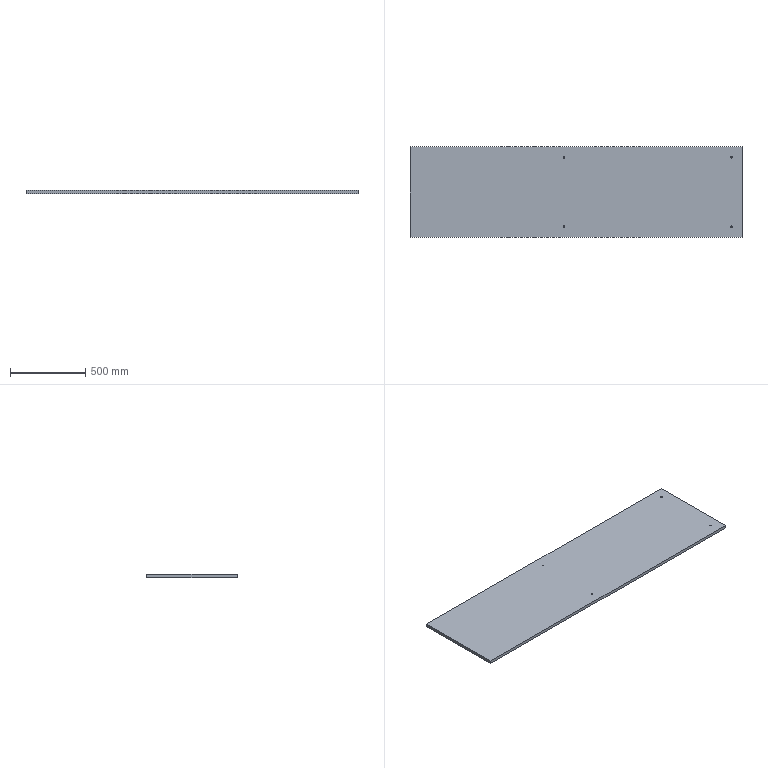Part | STEP file | B1-003 | 1 solid | 14 faces | box 2200 x 600 x 20 mm | volume 26393073 mm3 | cylinder 8 | plane 6 | commonest cylinder face diameters 10.5 x8
STEP:
#1=CARTESIAN_POINT('',(0.,0.,0.));
#2=DIRECTION('',(0.,0.,1.));
#3=DIRECTION('',(1.,0.,0.));
#4=AXIS2_PLACEMENT_3D('',#1,#2,#3);
#5=CARTESIAN_POINT('',(-85.25,230.,10.));
#6=VERTEX_POINT('',#5);
#7=CARTESIAN_POINT('',(-85.25,230.,-10.));
#8=VERTEX_POINT('',#7);
#9=CARTESIAN_POINT('',(-85.25,230.,24.849));
#10=DIRECTION('',(0.,0.,-1.));
#11=VECTOR('',#10,1.);
#12=LINE('',#9,#11);
#13=CARTESIAN_POINT('',(-80.,230.,24.849));
#14=DIRECTION('',(0.,0.,-1.));
#15=DIRECTION('',(-1.,0.,0.));
#16=AXIS2_PLACEMENT_3D('',#13,#14,#15);
#17=CYLINDRICAL_SURFACE('',#16,5.25);
#18=CARTESIAN_POINT('',(6.283,0.));
#19=DIRECTION('',(0.,1.));
#20=VECTOR('',#19,1.);
#21=LINE('',#18,#20);
#22=(GEOMETRIC_REPRESENTATION_CONTEXT(2)PARAMETRIC_REPRESENTATION_CONTEXT()REPRESENTATION_CONTEXT('',''));
#23=DEFINITIONAL_REPRESENTATION('',(#21),#22);
#24=PCURVE('',#17,#23);
#25=CARTESIAN_POINT('',(-80.,230.,24.849));
#26=DIRECTION('',(0.,0.,-1.));
#27=DIRECTION('',(-1.,0.,0.));
#28=AXIS2_PLACEMENT_3D('',#25,#26,#27);
#29=CYLINDRICAL_SURFACE('',#28,5.25);
#30=CARTESIAN_POINT('',(0.,0.));
#31=DIRECTION('',(0.,1.));
#32=VECTOR('',#31,1.);
#33=LINE('',#30,#32);
#34=(GEOMETRIC_REPRESENTATION_CONTEXT(2)PARAMETRIC_REPRESENTATION_CONTEXT()REPRESENTATION_CONTEXT('',''));
#35=DEFINITIONAL_REPRESENTATION('',(#33),#34);
#36=PCURVE('',#29,#35);
#37=SURFACE_CURVE('',#12,(#24,#36),.PCURVE_S1.);
#38=EDGE_CURVE('',#6,#8,#37,.T.);
#39=ORIENTED_EDGE('',*,*,#38,.T.);
#40=CARTESIAN_POINT('',(-74.75,230.,-10.));
#41=VERTEX_POINT('',#40);
#42=CARTESIAN_POINT('',(-80.,230.,-10.));
#43=DIRECTION('',(0.,0.,-1.));
#44=DIRECTION('',(-1.,0.,0.));
#45=AXIS2_PLACEMENT_3D('',#42,#43,#44);
#46=CIRCLE('',#45,5.25);
#47=CARTESIAN_POINT('',(0.,34.849));
#48=DIRECTION('',(1.,0.));
#49=VECTOR('',#48,1.);
#50=LINE('',#47,#49);
#51=(GEOMETRIC_REPRESENTATION_CONTEXT(2)PARAMETRIC_REPRESENTATION_CONTEXT()REPRESENTATION_CONTEXT('',''));
#52=DEFINITIONAL_REPRESENTATION('',(#50),#51);
#53=PCURVE('',#17,#52);
#54=CARTESIAN_POINT('',(0.,0.,-10.));
#55=DIRECTION('',(0.,0.,1.));
#56=DIRECTION('',(1.,0.,0.));
#57=AXIS2_PLACEMENT_3D('',#54,#55,#56);
#58=PLANE('',#57);
#59=CARTESIAN_POINT('',(-85.25,230.));
#60=CARTESIAN_POINT('',(-85.25,239.093));
#61=CARTESIAN_POINT('',(-77.375,234.547));
#62=CARTESIAN_POINT('',(-69.5,230.));
#63=CARTESIAN_POINT('',(-77.375,225.453));
#64=CARTESIAN_POINT('',(-85.25,220.907));
#65=CARTESIAN_POINT('',(-85.25,230.));
#66=(BOUNDED_CURVE()B_SPLINE_CURVE(2,(#59,#60,#61,#62,#63,#64,#65),.UNSPECIFIED.,.T.,.F.)B_SPLINE_CURVE_WITH_KNOTS((1,2,2,2,2,1),(-2.094,0.,2.094,4.189,6.283,8.378),.UNSPECIFIED.)CURVE()GEOMETRIC_REPRESENTATION_ITEM()RATIONAL_B_SPLINE_CURVE((1.,0.5,1.,0.5,1.,0.5,1.))REPRESENTATION_ITEM(''));
#67=(GEOMETRIC_REPRESENTATION_CONTEXT(2)PARAMETRIC_REPRESENTATION_CONTEXT()REPRESENTATION_CONTEXT('',''));
#68=DEFINITIONAL_REPRESENTATION('',(#66),#67);
#69=PCURVE('',#58,#68);
#70=SURFACE_CURVE('',#46,(#53,#69),.PCURVE_S1.);
#71=EDGE_CURVE('',#41,#8,#70,.T.);
#72=ORIENTED_EDGE('',*,*,#71,.F.);
#73=CARTESIAN_POINT('',(-74.75,230.,10.));
#74=VERTEX_POINT('',#73);
#75=CARTESIAN_POINT('',(-74.75,230.,24.849));
#76=DIRECTION('',(0.,0.,-1.));
#77=VECTOR('',#76,1.);
#78=LINE('',#75,#77);
#79=CARTESIAN_POINT('',(3.142,0.));
#80=DIRECTION('',(0.,1.));
#81=VECTOR('',#80,1.);
#82=LINE('',#79,#81);
#83=(GEOMETRIC_REPRESENTATION_CONTEXT(2)PARAMETRIC_REPRESENTATION_CONTEXT()REPRESENTATION_CONTEXT('',''));
#84=DEFINITIONAL_REPRESENTATION('',(#82),#83);
#85=PCURVE('',#17,#84);
#86=CARTESIAN_POINT('',(3.142,0.));
#87=DIRECTION('',(0.,1.));
#88=VECTOR('',#87,1.);
#89=LINE('',#86,#88);
#90=(GEOMETRIC_REPRESENTATION_CONTEXT(2)PARAMETRIC_REPRESENTATION_CONTEXT()REPRESENTATION_CONTEXT('',''));
#91=DEFINITIONAL_REPRESENTATION('',(#89),#90);
#92=PCURVE('',#29,#91);
#93=SURFACE_CURVE('',#78,(#85,#92),.PCURVE_S1.);
#94=EDGE_CURVE('',#74,#41,#93,.T.);
#95=ORIENTED_EDGE('',*,*,#94,.F.);
#96=CARTESIAN_POINT('',(-80.,230.,10.));
#97=DIRECTION('',(0.,0.,-1.));
#98=DIRECTION('',(1.,0.,0.));
#99=AXIS2_PLACEMENT_3D('',#96,#97,#98);
#100=CIRCLE('',#99,5.25);
#101=CARTESIAN_POINT('',(3.142,14.849));
#102=DIRECTION('',(1.,0.));
#103=VECTOR('',#102,1.);
#104=LINE('',#101,#103);
#105=(GEOMETRIC_REPRESENTATION_CONTEXT(2)PARAMETRIC_REPRESENTATION_CONTEXT()REPRESENTATION_CONTEXT('',''));
#106=DEFINITIONAL_REPRESENTATION('',(#104),#105);
#107=PCURVE('',#17,#106);
#108=CARTESIAN_POINT('',(0.,0.,10.));
#109=DIRECTION('',(0.,0.,1.));
#110=DIRECTION('',(1.,0.,0.));
#111=AXIS2_PLACEMENT_3D('',#108,#109,#110);
#112=PLANE('',#111);
#113=CARTESIAN_POINT('',(-74.75,230.));
#114=CARTESIAN_POINT('',(-74.75,220.907));
#115=CARTESIAN_POINT('',(-82.625,225.453));
#116=CARTESIAN_POINT('',(-90.5,230.));
#117=CARTESIAN_POINT('',(-82.625,234.547));
#118=CARTESIAN_POINT('',(-74.75,239.093));
#119=CARTESIAN_POINT('',(-74.75,230.));
#120=(BOUNDED_CURVE()B_SPLINE_CURVE(2,(#113,#114,#115,#116,#117,#118,#119),.UNSPECIFIED.,.T.,.F.)B_SPLINE_CURVE_WITH_KNOTS((1,2,2,2,2,1),(-2.094,0.,2.094,4.189,6.283,8.378),.UNSPECIFIED.)CURVE()GEOMETRIC_REPRESENTATION_ITEM()RATIONAL_B_SPLINE_CURVE((1.,0.5,1.,0.5,1.,0.5,1.))REPRESENTATION_ITEM(''));
#121=(GEOMETRIC_REPRESENTATION_CONTEXT(2)PARAMETRIC_REPRESENTATION_CONTEXT()REPRESENTATION_CONTEXT('',''));
#122=DEFINITIONAL_REPRESENTATION('',(#120),#121);
#123=PCURVE('',#112,#122);
#124=SURFACE_CURVE('',#100,(#107,#123),.PCURVE_S1.);
#125=EDGE_CURVE('',#74,#6,#124,.T.);
#126=ORIENTED_EDGE('',*,*,#125,.T.);
#127=EDGE_LOOP('',(#39,#72,#95,#126));
#128=FACE_BOUND('',#127,.F.);
#129=ADVANCED_FACE('',(#128),#17,.F.);
#130=CARTESIAN_POINT('',(1024.75,-230.,10.));
#131=VERTEX_POINT('',#130);
#132=CARTESIAN_POINT('',(1024.75,-230.,-10.));
#133=VERTEX_POINT('',#132);
#134=CARTESIAN_POINT('',(1024.75,-230.,24.849));
#135=DIRECTION('',(0.,0.,-1.));
#136=VECTOR('',#135,1.);
#137=LINE('',#134,#136);
#138=CARTESIAN_POINT('',(1030.,-230.,24.849));
#139=DIRECTION('',(0.,0.,-1.));
#140=DIRECTION('',(-1.,0.,0.));
#141=AXIS2_PLACEMENT_3D('',#138,#139,#140);
#142=CYLINDRICAL_SURFACE('',#141,5.25);
#143=CARTESIAN_POINT('',(6.283,0.));
#144=DIRECTION('',(0.,1.));
#145=VECTOR('',#144,1.);
#146=LINE('',#143,#145);
#147=(GEOMETRIC_REPRESENTATION_CONTEXT(2)PARAMETRIC_REPRESENTATION_CONTEXT()REPRESENTATION_CONTEXT('',''));
#148=DEFINITIONAL_REPRESENTATION('',(#146),#147);
#149=PCURVE('',#142,#148);
#150=CARTESIAN_POINT('',(1030.,-230.,24.849));
#151=DIRECTION('',(0.,0.,-1.));
#152=DIRECTION('',(-1.,0.,0.));
#153=AXIS2_PLACEMENT_3D('',#150,#151,#152);
#154=CYLINDRICAL_SURFACE('',#153,5.25);
#155=CARTESIAN_POINT('',(0.,0.));
#156=DIRECTION('',(0.,1.));
#157=VECTOR('',#156,1.);
#158=LINE('',#155,#157);
#159=(GEOMETRIC_REPRESENTATION_CONTEXT(2)PARAMETRIC_REPRESENTATION_CONTEXT()REPRESENTATION_CONTEXT('',''));
#160=DEFINITIONAL_REPRESENTATION('',(#158),#159);
#161=PCURVE('',#154,#160);
#162=SURFACE_CURVE('',#137,(#149,#161),.PCURVE_S1.);
#163=EDGE_CURVE('',#131,#133,#162,.T.);
#164=ORIENTED_EDGE('',*,*,#163,.T.);
#165=CARTESIAN_POINT('',(1035.25,-230.,-10.));
#166=VERTEX_POINT('',#165);
#167=CARTESIAN_POINT('',(1030.,-230.,-10.));
#168=DIRECTION('',(0.,0.,-1.));
#169=DIRECTION('',(-1.,0.,0.));
#170=AXIS2_PLACEMENT_3D('',#167,#168,#169);
#171=CIRCLE('',#170,5.25);
#172=CARTESIAN_POINT('',(0.,34.849));
#173=DIRECTION('',(1.,0.));
#174=VECTOR('',#173,1.);
#175=LINE('',#172,#174);
#176=(GEOMETRIC_REPRESENTATION_CONTEXT(2)PARAMETRIC_REPRESENTATION_CONTEXT()REPRESENTATION_CONTEXT('',''));
#177=DEFINITIONAL_REPRESENTATION('',(#175),#176);
#178=PCURVE('',#142,#177);
#179=CARTESIAN_POINT('',(1024.75,-230.));
#180=CARTESIAN_POINT('',(1024.75,-220.907));
#181=CARTESIAN_POINT('',(1032.625,-225.453));
#182=CARTESIAN_POINT('',(1040.5,-230.));
#183=CARTESIAN_POINT('',(1032.625,-234.547));
#184=CARTESIAN_POINT('',(1024.75,-239.093));
#185=CARTESIAN_POINT('',(1024.75,-230.));
#186=(BOUNDED_CURVE()B_SPLINE_CURVE(2,(#179,#180,#181,#182,#183,#184,#185),.UNSPECIFIED.,.T.,.F.)B_SPLINE_CURVE_WITH_KNOTS((1,2,2,2,2,1),(-2.094,0.,2.094,4.189,6.283,8.378),.UNSPECIFIED.)CURVE()GEOMETRIC_REPRESENTATION_ITEM()RATIONAL_B_SPLINE_CURVE((1.,0.5,1.,0.5,1.,0.5,1.))REPRESENTATION_ITEM(''));
#187=(GEOMETRIC_REPRESENTATION_CONTEXT(2)PARAMETRIC_REPRESENTATION_CONTEXT()REPRESENTATION_CONTEXT('',''));
#188=DEFINITIONAL_REPRESENTATION('',(#186),#187);
#189=PCURVE('',#58,#188);
#190=SURFACE_CURVE('',#171,(#178,#189),.PCURVE_S1.);
#191=EDGE_CURVE('',#166,#133,#190,.T.);
#192=ORIENTED_EDGE('',*,*,#191,.F.);
#193=CARTESIAN_POINT('',(1035.25,-230.,10.));
#194=VERTEX_POINT('',#193);
#195=CARTESIAN_POINT('',(1035.25,-230.,24.849));
#196=DIRECTION('',(0.,0.,-1.));
#197=VECTOR('',#196,1.);
#198=LINE('',#195,#197);
#199=CARTESIAN_POINT('',(3.142,0.));
#200=DIRECTION('',(0.,1.));
#201=VECTOR('',#200,1.);
#202=LINE('',#199,#201);
#203=(GEOMETRIC_REPRESENTATION_CONTEXT(2)PARAMETRIC_REPRESENTATION_CONTEXT()REPRESENTATION_CONTEXT('',''));
#204=DEFINITIONAL_REPRESENTATION('',(#202),#203);
#205=PCURVE('',#142,#204);
#206=CARTESIAN_POINT('',(3.142,0.));
#207=DIRECTION('',(0.,1.));
#208=VECTOR('',#207,1.);
#209=LINE('',#206,#208);
#210=(GEOMETRIC_REPRESENTATION_CONTEXT(2)PARAMETRIC_REPRESENTATION_CONTEXT()REPRESENTATION_CONTEXT('',''));
#211=DEFINITIONAL_REPRESENTATION('',(#209),#210);
#212=PCURVE('',#154,#211);
#213=SURFACE_CURVE('',#198,(#205,#212),.PCURVE_S1.);
#214=EDGE_CURVE('',#194,#166,#213,.T.);
#215=ORIENTED_EDGE('',*,*,#214,.F.);
#216=CARTESIAN_POINT('',(1030.,-230.,10.));
#217=DIRECTION('',(0.,0.,-1.));
#218=DIRECTION('',(1.,0.,0.));
#219=AXIS2_PLACEMENT_3D('',#216,#217,#218);
#220=CIRCLE('',#219,5.25);
#221=CARTESIAN_POINT('',(3.142,14.849));
#222=DIRECTION('',(1.,0.));
#223=VECTOR('',#222,1.);
#224=LINE('',#221,#223);
#225=(GEOMETRIC_REPRESENTATION_CONTEXT(2)PARAMETRIC_REPRESENTATION_CONTEXT()REPRESENTATION_CONTEXT('',''));
#226=DEFINITIONAL_REPRESENTATION('',(#224),#225);
#227=PCURVE('',#142,#226);
#228=CARTESIAN_POINT('',(1035.25,-230.));
#229=CARTESIAN_POINT('',(1035.25,-239.093));
#230=CARTESIAN_POINT('',(1027.375,-234.547));
#231=CARTESIAN_POINT('',(1019.5,-230.));
#232=CARTESIAN_POINT('',(1027.375,-225.453));
#233=CARTESIAN_POINT('',(1035.25,-220.907));
#234=CARTESIAN_POINT('',(1035.25,-230.));
#235=(BOUNDED_CURVE()B_SPLINE_CURVE(2,(#228,#229,#230,#231,#232,#233,#234),.UNSPECIFIED.,.T.,.F.)B_SPLINE_CURVE_WITH_KNOTS((1,2,2,2,2,1),(-2.094,0.,2.094,4.189,6.283,8.378),.UNSPECIFIED.)CURVE()GEOMETRIC_REPRESENTATION_ITEM()RATIONAL_B_SPLINE_CURVE((1.,0.5,1.,0.5,1.,0.5,1.))REPRESENTATION_ITEM(''));
#236=(GEOMETRIC_REPRESENTATION_CONTEXT(2)PARAMETRIC_REPRESENTATION_CONTEXT()REPRESENTATION_CONTEXT('',''));
#237=DEFINITIONAL_REPRESENTATION('',(#235),#236);
#238=PCURVE('',#112,#237);
#239=SURFACE_CURVE('',#220,(#227,#238),.PCURVE_S1.);
#240=EDGE_CURVE('',#194,#131,#239,.T.);
#241=ORIENTED_EDGE('',*,*,#240,.T.);
#242=EDGE_LOOP('',(#164,#192,#215,#241));
#243=FACE_BOUND('',#242,.F.);
#244=ADVANCED_FACE('',(#243),#142,.F.);
#245=CARTESIAN_POINT('',(1024.75,230.,10.));
#246=VERTEX_POINT('',#245);
#247=CARTESIAN_POINT('',(1024.75,230.,-10.));
#248=VERTEX_POINT('',#247);
#249=CARTESIAN_POINT('',(1024.75,230.,24.849));
#250=DIRECTION('',(0.,0.,-1.));
#251=VECTOR('',#250,1.);
#252=LINE('',#249,#251);
#253=CARTESIAN_POINT('',(1030.,230.,24.849));
#254=DIRECTION('',(0.,0.,-1.));
#255=DIRECTION('',(-1.,0.,0.));
#256=AXIS2_PLACEMENT_3D('',#253,#254,#255);
#257=CYLINDRICAL_SURFACE('',#256,5.25);
#258=CARTESIAN_POINT('',(6.283,0.));
#259=DIRECTION('',(0.,1.));
#260=VECTOR('',#259,1.);
#261=LINE('',#258,#260);
#262=(GEOMETRIC_REPRESENTATION_CONTEXT(2)PARAMETRIC_REPRESENTATION_CONTEXT()REPRESENTATION_CONTEXT('',''));
#263=DEFINITIONAL_REPRESENTATION('',(#261),#262);
#264=PCURVE('',#257,#263);
#265=CARTESIAN_POINT('',(1030.,230.,24.849));
#266=DIRECTION('',(0.,0.,-1.));
#267=DIRECTION('',(-1.,0.,0.));
#268=AXIS2_PLACEMENT_3D('',#265,#266,#267);
#269=CYLINDRICAL_SURFACE('',#268,5.25);
#270=CARTESIAN_POINT('',(0.,0.));
#271=DIRECTION('',(0.,1.));
#272=VECTOR('',#271,1.);
#273=LINE('',#270,#272);
#274=(GEOMETRIC_REPRESENTATION_CONTEXT(2)PARAMETRIC_REPRESENTATION_CONTEXT()REPRESENTATION_CONTEXT('',''));
#275=DEFINITIONAL_REPRESENTATION('',(#273),#274);
#276=PCURVE('',#269,#275);
#277=SURFACE_CURVE('',#252,(#264,#276),.PCURVE_S1.);
#278=EDGE_CURVE('',#246,#248,#277,.T.);
#279=ORIENTED_EDGE('',*,*,#278,.T.);
#280=CARTESIAN_POINT('',(1035.25,230.,-10.));
#281=VERTEX_POINT('',#280);
#282=CARTESIAN_POINT('',(1030.,230.,-10.));
#283=DIRECTION('',(0.,0.,-1.));
#284=DIRECTION('',(-1.,0.,0.));
#285=AXIS2_PLACEMENT_3D('',#282,#283,#284);
#286=CIRCLE('',#285,5.25);
#287=CARTESIAN_POINT('',(0.,34.849));
#288=DIRECTION('',(1.,0.));
#289=VECTOR('',#288,1.);
#290=LINE('',#287,#289);
#291=(GEOMETRIC_REPRESENTATION_CONTEXT(2)PARAMETRIC_REPRESENTATION_CONTEXT()REPRESENTATION_CONTEXT('',''));
#292=DEFINITIONAL_REPRESENTATION('',(#290),#291);
#293=PCURVE('',#257,#292);
#294=CARTESIAN_POINT('',(1024.75,230.));
#295=CARTESIAN_POINT('',(1024.75,239.093));
#296=CARTESIAN_POINT('',(1032.625,234.547));
#297=CARTESIAN_POINT('',(1040.5,230.));
#298=CARTESIAN_POINT('',(1032.625,225.453));
#299=CARTESIAN_POINT('',(1024.75,220.907));
#300=CARTESIAN_POINT('',(1024.75,230.));
#301=(BOUNDED_CURVE()B_SPLINE_CURVE(2,(#294,#295,#296,#297,#298,#299,#300),.UNSPECIFIED.,.T.,.F.)B_SPLINE_CURVE_WITH_KNOTS((1,2,2,2,2,1),(-2.094,0.,2.094,4.189,6.283,8.378),.UNSPECIFIED.)CURVE()GEOMETRIC_REPRESENTATION_ITEM()RATIONAL_B_SPLINE_CURVE((1.,0.5,1.,0.5,1.,0.5,1.))REPRESENTATION_ITEM(''));
#302=(GEOMETRIC_REPRESENTATION_CONTEXT(2)PARAMETRIC_REPRESENTATION_CONTEXT()REPRESENTATION_CONTEXT('',''));
#303=DEFINITIONAL_REPRESENTATION('',(#301),#302);
#304=PCURVE('',#58,#303);
#305=SURFACE_CURVE('',#286,(#293,#304),.PCURVE_S1.);
#306=EDGE_CURVE('',#281,#248,#305,.T.);
#307=ORIENTED_EDGE('',*,*,#306,.F.);
#308=CARTESIAN_POINT('',(1035.25,230.,10.));
#309=VERTEX_POINT('',#308);
#310=CARTESIAN_POINT('',(1035.25,230.,24.849));
#311=DIRECTION('',(0.,0.,-1.));
#312=VECTOR('',#311,1.);
#313=LINE('',#310,#312);
#314=CARTESIAN_POINT('',(3.142,0.));
#315=DIRECTION('',(0.,1.));
#316=VECTOR('',#315,1.);
#317=LINE('',#314,#316);
#318=(GEOMETRIC_REPRESENTATION_CONTEXT(2)PARAMETRIC_REPRESENTATION_CONTEXT()REPRESENTATION_CONTEXT('',''));
#319=DEFINITIONAL_REPRESENTATION('',(#317),#318);
#320=PCURVE('',#257,#319);
#321=CARTESIAN_POINT('',(3.142,0.));
#322=DIRECTION('',(0.,1.));
#323=VECTOR('',#322,1.);
#324=LINE('',#321,#323);
#325=(GEOMETRIC_REPRESENTATION_CONTEXT(2)PARAMETRIC_REPRESENTATION_CONTEXT()REPRESENTATION_CONTEXT('',''));
#326=DEFINITIONAL_REPRESENTATION('',(#324),#325);
#327=PCURVE('',#269,#326);
#328=SURFACE_CURVE('',#313,(#320,#327),.PCURVE_S1.);
#329=EDGE_CURVE('',#309,#281,#328,.T.);
#330=ORIENTED_EDGE('',*,*,#329,.F.);
#331=CARTESIAN_POINT('',(1030.,230.,10.));
#332=DIRECTION('',(0.,0.,-1.));
#333=DIRECTION('',(1.,0.,0.));
#334=AXIS2_PLACEMENT_3D('',#331,#332,#333);
#335=CIRCLE('',#334,5.25);
#336=CARTESIAN_POINT('',(3.142,14.849));
#337=DIRECTION('',(1.,0.));
#338=VECTOR('',#337,1.);
#339=LINE('',#336,#338);
#340=(GEOMETRIC_REPRESENTATION_CONTEXT(2)PARAMETRIC_REPRESENTATION_CONTEXT()REPRESENTATION_CONTEXT('',''));
#341=DEFINITIONAL_REPRESENTATION('',(#339),#340);
#342=PCURVE('',#257,#341);
#343=CARTESIAN_POINT('',(1035.25,230.));
#344=CARTESIAN_POINT('',(1035.25,220.907));
#345=CARTESIAN_POINT('',(1027.375,225.453));
#346=CARTESIAN_POINT('',(1019.5,230.));
#347=CARTESIAN_POINT('',(1027.375,234.547));
#348=CARTESIAN_POINT('',(1035.25,239.093));
#349=CARTESIAN_POINT('',(1035.25,230.));
#350=(BOUNDED_CURVE()B_SPLINE_CURVE(2,(#343,#344,#345,#346,#347,#348,#349),.UNSPECIFIED.,.T.,.F.)B_SPLINE_CURVE_WITH_KNOTS((1,2,2,2,2,1),(-2.094,0.,2.094,4.189,6.283,8.378),.UNSPECIFIED.)CURVE()GEOMETRIC_REPRESENTATION_ITEM()RATIONAL_B_SPLINE_CURVE((1.,0.5,1.,0.5,1.,0.5,1.))REPRESENTATION_ITEM(''));
#351=(GEOMETRIC_REPRESENTATION_CONTEXT(2)PARAMETRIC_REPRESENTATION_CONTEXT()REPRESENTATION_CONTEXT('',''));
#352=DEFINITIONAL_REPRESENTATION('',(#350),#351);
#353=PCURVE('',#112,#352);
#354=SURFACE_CURVE('',#335,(#342,#353),.PCURVE_S1.);
#355=EDGE_CURVE('',#309,#246,#354,.T.);
#356=ORIENTED_EDGE('',*,*,#355,.T.);
#357=EDGE_LOOP('',(#279,#307,#330,#356));
#358=FACE_BOUND('',#357,.F.);
#359=ADVANCED_FACE('',(#358),#257,.F.);
#360=CARTESIAN_POINT('',(-85.25,-230.,10.));
#361=VERTEX_POINT('',#360);
#362=CARTESIAN_POINT('',(-85.25,-230.,-10.));
#363=VERTEX_POINT('',#362);
#364=CARTESIAN_POINT('',(-85.25,-230.,24.849));
#365=DIRECTION('',(0.,0.,-1.));
#366=VECTOR('',#365,1.);
#367=LINE('',#364,#366);
#368=CARTESIAN_POINT('',(-80.,-230.,24.849));
#369=DIRECTION('',(0.,0.,-1.));
#370=DIRECTION('',(-1.,0.,0.));
#371=AXIS2_PLACEMENT_3D('',#368,#369,#370);
#372=CYLINDRICAL_SURFACE('',#371,5.25);
#373=CARTESIAN_POINT('',(6.283,0.));
#374=DIRECTION('',(0.,1.));
#375=VECTOR('',#374,1.);
#376=LINE('',#373,#375);
#377=(GEOMETRIC_REPRESENTATION_CONTEXT(2)PARAMETRIC_REPRESENTATION_CONTEXT()REPRESENTATION_CONTEXT('',''));
#378=DEFINITIONAL_REPRESENTATION('',(#376),#377);
#379=PCURVE('',#372,#378);
#380=CARTESIAN_POINT('',(-80.,-230.,24.849));
#381=DIRECTION('',(0.,0.,-1.));
#382=DIRECTION('',(-1.,0.,0.));
#383=AXIS2_PLACEMENT_3D('',#380,#381,#382);
#384=CYLINDRICAL_SURFACE('',#383,5.25);
#385=CARTESIAN_POINT('',(0.,0.));
#386=DIRECTION('',(0.,1.));
#387=VECTOR('',#386,1.);
#388=LINE('',#385,#387);
#389=(GEOMETRIC_REPRESENTATION_CONTEXT(2)PARAMETRIC_REPRESENTATION_CONTEXT()REPRESENTATION_CONTEXT('',''));
#390=DEFINITIONAL_REPRESENTATION('',(#388),#389);
#391=PCURVE('',#384,#390);
#392=SURFACE_CURVE('',#367,(#379,#391),.PCURVE_S1.);
#393=EDGE_CURVE('',#361,#363,#392,.T.);
#394=ORIENTED_EDGE('',*,*,#393,.T.);
#395=CARTESIAN_POINT('',(-74.75,-230.,-10.));
#396=VERTEX_POINT('',#395);
#397=CARTESIAN_POINT('',(-80.,-230.,-10.));
#398=DIRECTION('',(0.,0.,-1.));
#399=DIRECTION('',(-1.,0.,0.));
#400=AXIS2_PLACEMENT_3D('',#397,#398,#399);
#401=CIRCLE('',#400,5.25);
#402=CARTESIAN_POINT('',(0.,34.849));
#403=DIRECTION('',(1.,0.));
#404=VECTOR('',#403,1.);
#405=LINE('',#402,#404);
#406=(GEOMETRIC_REPRESENTATION_CONTEXT(2)PARAMETRIC_REPRESENTATION_CONTEXT()REPRESENTATION_CONTEXT('',''));
#407=DEFINITIONAL_REPRESENTATION('',(#405),#406);
#408=PCURVE('',#372,#407);
#409=CARTESIAN_POINT('',(-85.25,-230.));
#410=CARTESIAN_POINT('',(-85.25,-220.907));
#411=CARTESIAN_POINT('',(-77.375,-225.453));
#412=CARTESIAN_POINT('',(-69.5,-230.));
#413=CARTESIAN_POINT('',(-77.375,-234.547));
#414=CARTESIAN_POINT('',(-85.25,-239.093));
#415=CARTESIAN_POINT('',(-85.25,-230.));
#416=(BOUNDED_CURVE()B_SPLINE_CURVE(2,(#409,#410,#411,#412,#413,#414,#415),.UNSPECIFIED.,.T.,.F.)B_SPLINE_CURVE_WITH_KNOTS((1,2,2,2,2,1),(-2.094,0.,2.094,4.189,6.283,8.378),.UNSPECIFIED.)CURVE()GEOMETRIC_REPRESENTATION_ITEM()RATIONAL_B_SPLINE_CURVE((1.,0.5,1.,0.5,1.,0.5,1.))REPRESENTATION_ITEM(''));
#417=(GEOMETRIC_REPRESENTATION_CONTEXT(2)PARAMETRIC_REPRESENTATION_CONTEXT()REPRESENTATION_CONTEXT('',''));
#418=DEFINITIONAL_REPRESENTATION('',(#416),#417);
#419=PCURVE('',#58,#418);
#420=SURFACE_CURVE('',#401,(#408,#419),.PCURVE_S1.);
#421=EDGE_CURVE('',#396,#363,#420,.T.);
#422=ORIENTED_EDGE('',*,*,#421,.F.);
#423=CARTESIAN_POINT('',(-74.75,-230.,10.));
#424=VERTEX_POINT('',#423);
#425=CARTESIAN_POINT('',(-74.75,-230.,24.849));
#426=DIRECTION('',(0.,0.,-1.));
#427=VECTOR('',#426,1.);
#428=LINE('',#425,#427);
#429=CARTESIAN_POINT('',(3.142,0.));
#430=DIRECTION('',(0.,1.));
#431=VECTOR('',#430,1.);
#432=LINE('',#429,#431);
#433=(GEOMETRIC_REPRESENTATION_CONTEXT(2)PARAMETRIC_REPRESENTATION_CONTEXT()REPRESENTATION_CONTEXT('',''));
#434=DEFINITIONAL_REPRESENTATION('',(#432),#433);
#435=PCURVE('',#372,#434);
#436=CARTESIAN_POINT('',(3.142,0.));
#437=DIRECTION('',(0.,1.));
#438=VECTOR('',#437,1.);
#439=LINE('',#436,#438);
#440=(GEOMETRIC_REPRESENTATION_CONTEXT(2)PARAMETRIC_REPRESENTATION_CONTEXT()REPRESENTATION_CONTEXT('',''));
#441=DEFINITIONAL_REPRESENTATION('',(#439),#440);
#442=PCURVE('',#384,#441);
#443=SURFACE_CURVE('',#428,(#435,#442),.PCURVE_S1.);
#444=EDGE_CURVE('',#424,#396,#443,.T.);
#445=ORIENTED_EDGE('',*,*,#444,.F.);
#446=CARTESIAN_POINT('',(-80.,-230.,10.));
#447=DIRECTION('',(0.,0.,-1.));
#448=DIRECTION('',(1.,0.,0.));
#449=AXIS2_PLACEMENT_3D('',#446,#447,#448);
#450=CIRCLE('',#449,5.25);
#451=CARTESIAN_POINT('',(3.142,14.849));
#452=DIRECTION('',(1.,0.));
#453=VECTOR('',#452,1.);
#454=LINE('',#451,#453);
#455=(GEOMETRIC_REPRESENTATION_CONTEXT(2)PARAMETRIC_REPRESENTATION_CONTEXT()REPRESENTATION_CONTEXT('',''));
#456=DEFINITIONAL_REPRESENTATION('',(#454),#455);
#457=PCURVE('',#372,#456);
#458=CARTESIAN_POINT('',(-74.75,-230.));
#459=CARTESIAN_POINT('',(-74.75,-239.093));
#460=CARTESIAN_POINT('',(-82.625,-234.547));
#461=CARTESIAN_POINT('',(-90.5,-230.));
#462=CARTESIAN_POINT('',(-82.625,-225.453));
#463=CARTESIAN_POINT('',(-74.75,-220.907));
#464=CARTESIAN_POINT('',(-74.75,-230.));
#465=(BOUNDED_CURVE()B_SPLINE_CURVE(2,(#458,#459,#460,#461,#462,#463,#464),.UNSPECIFIED.,.T.,.F.)B_SPLINE_CURVE_WITH_KNOTS((1,2,2,2,2,1),(-2.094,0.,2.094,4.189,6.283,8.378),.UNSPECIFIED.)CURVE()GEOMETRIC_REPRESENTATION_ITEM()RATIONAL_B_SPLINE_CURVE((1.,0.5,1.,0.5,1.,0.5,1.))REPRESENTATION_ITEM(''));
#466=(GEOMETRIC_REPRESENTATION_CONTEXT(2)PARAMETRIC_REPRESENTATION_CONTEXT()REPRESENTATION_CONTEXT('',''));
#467=DEFINITIONAL_REPRESENTATION('',(#465),#466);
#468=PCURVE('',#112,#467);
#469=SURFACE_CURVE('',#450,(#457,#468),.PCURVE_S1.);
#470=EDGE_CURVE('',#424,#361,#469,.T.);
#471=ORIENTED_EDGE('',*,*,#470,.T.);
#472=EDGE_LOOP('',(#394,#422,#445,#471));
#473=FACE_BOUND('',#472,.F.);
#474=ADVANCED_FACE('',(#473),#372,.F.);
#475=CARTESIAN_POINT('',(1100.,-300.,-10.));
#476=VERTEX_POINT('',#475);
#477=CARTESIAN_POINT('',(1100.,300.,-10.));
#478=VERTEX_POINT('',#477);
#479=CARTESIAN_POINT('',(1100.,300.,-10.));
#480=DIRECTION('',(0.,1.,0.));
#481=VECTOR('',#480,1.);
#482=LINE('',#479,#481);
#483=CARTESIAN_POINT('',(1100.,300.,10.));
#484=DIRECTION('',(-1.,0.,0.));
#485=DIRECTION('',(0.,0.,1.));
#486=AXIS2_PLACEMENT_3D('',#483,#484,#485);
#487=PLANE('',#486);
#488=CARTESIAN_POINT('',(-20.,0.));
#489=DIRECTION('',(0.,1.));
#490=VECTOR('',#489,1.);
#491=LINE('',#488,#490);
#492=(GEOMETRIC_REPRESENTATION_CONTEXT(2)PARAMETRIC_REPRESENTATION_CONTEXT()REPRESENTATION_CONTEXT('',''));
#493=DEFINITIONAL_REPRESENTATION('',(#491),#492);
#494=PCURVE('',#487,#493);
#495=CARTESIAN_POINT('',(1100.,300.));
#496=DIRECTION('',(0.,1.));
#497=VECTOR('',#496,1.);
#498=LINE('',#495,#497);
#499=(GEOMETRIC_REPRESENTATION_CONTEXT(2)PARAMETRIC_REPRESENTATION_CONTEXT()REPRESENTATION_CONTEXT('',''));
#500=DEFINITIONAL_REPRESENTATION('',(#498),#499);
#501=PCURVE('',#58,#500);
#502=SURFACE_CURVE('',#482,(#494,#501),.PCURVE_S1.);
#503=EDGE_CURVE('',#476,#478,#502,.T.);
#504=ORIENTED_EDGE('',*,*,#503,.T.);
#505=CARTESIAN_POINT('',(1100.,300.,10.));
#506=VERTEX_POINT('',#505);
#507=CARTESIAN_POINT('',(1100.,300.,10.));
#508=DIRECTION('',(0.,0.,-1.));
#509=VECTOR('',#508,1.);
#510=LINE('',#507,#509);
#511=CARTESIAN_POINT('',(0.,0.));
#512=DIRECTION('',(-1.,0.));
#513=VECTOR('',#512,1.);
#514=LINE('',#511,#513);
#515=(GEOMETRIC_REPRESENTATION_CONTEXT(2)PARAMETRIC_REPRESENTATION_CONTEXT()REPRESENTATION_CONTEXT('',''));
#516=DEFINITIONAL_REPRESENTATION('',(#514),#515);
#517=PCURVE('',#487,#516);
#518=CARTESIAN_POINT('',(-1100.,300.,10.));
#519=DIRECTION('',(0.,-1.,0.));
#520=DIRECTION('',(0.,0.,-1.));
#521=AXIS2_PLACEMENT_3D('',#518,#519,#520);
#522=PLANE('',#521);
#523=CARTESIAN_POINT('',(0.,2200.));
#524=DIRECTION('',(1.,0.));
#525=VECTOR('',#524,1.);
#526=LINE('',#523,#525);
#527=(GEOMETRIC_REPRESENTATION_CONTEXT(2)PARAMETRIC_REPRESENTATION_CONTEXT()REPRESENTATION_CONTEXT('',''));
#528=DEFINITIONAL_REPRESENTATION('',(#526),#527);
#529=PCURVE('',#522,#528);
#530=SURFACE_CURVE('',#510,(#517,#529),.PCURVE_S1.);
#531=EDGE_CURVE('',#506,#478,#530,.T.);
#532=ORIENTED_EDGE('',*,*,#531,.F.);
#533=CARTESIAN_POINT('',(1100.,-300.,10.));
#534=VERTEX_POINT('',#533);
#535=CARTESIAN_POINT('',(1100.,300.,10.));
#536=DIRECTION('',(0.,1.,0.));
#537=VECTOR('',#536,1.);
#538=LINE('',#535,#537);
#539=CARTESIAN_POINT('',(0.,0.));
#540=DIRECTION('',(0.,1.));
#541=VECTOR('',#540,1.);
#542=LINE('',#539,#541);
#543=(GEOMETRIC_REPRESENTATION_CONTEXT(2)PARAMETRIC_REPRESENTATION_CONTEXT()REPRESENTATION_CONTEXT('',''));
#544=DEFINITIONAL_REPRESENTATION('',(#542),#543);
#545=PCURVE('',#487,#544);
#546=CARTESIAN_POINT('',(1100.,300.));
#547=DIRECTION('',(0.,1.));
#548=VECTOR('',#547,1.);
#549=LINE('',#546,#548);
#550=(GEOMETRIC_REPRESENTATION_CONTEXT(2)PARAMETRIC_REPRESENTATION_CONTEXT()REPRESENTATION_CONTEXT('',''));
#551=DEFINITIONAL_REPRESENTATION('',(#549),#550);
#552=PCURVE('',#112,#551);
#553=SURFACE_CURVE('',#538,(#545,#552),.PCURVE_S1.);
#554=EDGE_CURVE('',#534,#506,#553,.T.);
#555=ORIENTED_EDGE('',*,*,#554,.F.);
#556=CARTESIAN_POINT('',(1100.,-300.,10.));
#557=DIRECTION('',(0.,0.,-1.));
#558=VECTOR('',#557,1.);
#559=LINE('',#556,#558);
#560=CARTESIAN_POINT('',(0.,-600.));
#561=DIRECTION('',(-1.,0.));
#562=VECTOR('',#561,1.);
#563=LINE('',#560,#562);
#564=(GEOMETRIC_REPRESENTATION_CONTEXT(2)PARAMETRIC_REPRESENTATION_CONTEXT()REPRESENTATION_CONTEXT('',''));
#565=DEFINITIONAL_REPRESENTATION('',(#563),#564);
#566=PCURVE('',#487,#565);
#567=CARTESIAN_POINT('',(-1100.,-300.,10.));
#568=DIRECTION('',(0.,1.,0.));
#569=DIRECTION('',(0.,0.,1.));
#570=AXIS2_PLACEMENT_3D('',#567,#568,#569);
#571=PLANE('',#570);
#572=CARTESIAN_POINT('',(0.,2200.));
#573=DIRECTION('',(-1.,0.));
#574=VECTOR('',#573,1.);
#575=LINE('',#572,#574);
#576=(GEOMETRIC_REPRESENTATION_CONTEXT(2)PARAMETRIC_REPRESENTATION_CONTEXT()REPRESENTATION_CONTEXT('',''));
#577=DEFINITIONAL_REPRESENTATION('',(#575),#576);
#578=PCURVE('',#571,#577);
#579=SURFACE_CURVE('',#559,(#566,#578),.PCURVE_S1.);
#580=EDGE_CURVE('',#534,#476,#579,.T.);
#581=ORIENTED_EDGE('',*,*,#580,.T.);
#582=EDGE_LOOP('',(#504,#532,#555,#581));
#583=FACE_BOUND('',#582,.T.);
#584=ADVANCED_FACE('',(#583),#487,.F.);
#585=CARTESIAN_POINT('',(-1100.,300.,-10.));
#586=VERTEX_POINT('',#585);
#587=CARTESIAN_POINT('',(-1100.,300.,-10.));
#588=DIRECTION('',(-1.,0.,0.));
#589=VECTOR('',#588,1.);
#590=LINE('',#587,#589);
#591=CARTESIAN_POINT('',(20.,0.));
#592=DIRECTION('',(0.,-1.));
#593=VECTOR('',#592,1.);
#594=LINE('',#591,#593);
#595=(GEOMETRIC_REPRESENTATION_CONTEXT(2)PARAMETRIC_REPRESENTATION_CONTEXT()REPRESENTATION_CONTEXT('',''));
#596=DEFINITIONAL_REPRESENTATION('',(#594),#595);
#597=PCURVE('',#522,#596);
#598=CARTESIAN_POINT('',(-1100.,300.));
#599=DIRECTION('',(-1.,0.));
#600=VECTOR('',#599,1.);
#601=LINE('',#598,#600);
#602=(GEOMETRIC_REPRESENTATION_CONTEXT(2)PARAMETRIC_REPRESENTATION_CONTEXT()REPRESENTATION_CONTEXT('',''));
#603=DEFINITIONAL_REPRESENTATION('',(#601),#602);
#604=PCURVE('',#58,#603);
#605=SURFACE_CURVE('',#590,(#597,#604),.PCURVE_S1.);
#606=EDGE_CURVE('',#478,#586,#605,.T.);
#607=ORIENTED_EDGE('',*,*,#606,.T.);
#608=CARTESIAN_POINT('',(-1100.,300.,10.));
#609=VERTEX_POINT('',#608);
#610=CARTESIAN_POINT('',(-1100.,300.,10.));
#611=DIRECTION('',(0.,0.,-1.));
#612=VECTOR('',#611,1.);
#613=LINE('',#610,#612);
#614=CARTESIAN_POINT('',(0.,0.));
#615=DIRECTION('',(1.,0.));
#616=VECTOR('',#615,1.);
#617=LINE('',#614,#616);
#618=(GEOMETRIC_REPRESENTATION_CONTEXT(2)PARAMETRIC_REPRESENTATION_CONTEXT()REPRESENTATION_CONTEXT('',''));
#619=DEFINITIONAL_REPRESENTATION('',(#617),#618);
#620=PCURVE('',#522,#619);
#621=CARTESIAN_POINT('',(-1100.,300.,10.));
#622=DIRECTION('',(1.,0.,0.));
#623=DIRECTION('',(0.,0.,-1.));
#624=AXIS2_PLACEMENT_3D('',#621,#622,#623);
#625=PLANE('',#624);
#626=CARTESIAN_POINT('',(0.,0.));
#627=DIRECTION('',(1.,0.));
#628=VECTOR('',#627,1.);
#629=LINE('',#626,#628);
#630=(GEOMETRIC_REPRESENTATION_CONTEXT(2)PARAMETRIC_REPRESENTATION_CONTEXT()REPRESENTATION_CONTEXT('',''));
#631=DEFINITIONAL_REPRESENTATION('',(#629),#630);
#632=PCURVE('',#625,#631);
#633=SURFACE_CURVE('',#613,(#620,#632),.PCURVE_S1.);
#634=EDGE_CURVE('',#609,#586,#633,.T.);
#635=ORIENTED_EDGE('',*,*,#634,.F.);
#636=CARTESIAN_POINT('',(-1100.,300.,10.));
#637=DIRECTION('',(-1.,0.,0.));
#638=VECTOR('',#637,1.);
#639=LINE('',#636,#638);
#640=CARTESIAN_POINT('',(0.,0.));
#641=DIRECTION('',(0.,-1.));
#642=VECTOR('',#641,1.);
#643=LINE('',#640,#642);
#644=(GEOMETRIC_REPRESENTATION_CONTEXT(2)PARAMETRIC_REPRESENTATION_CONTEXT()REPRESENTATION_CONTEXT('',''));
#645=DEFINITIONAL_REPRESENTATION('',(#643),#644);
#646=PCURVE('',#522,#645);
#647=CARTESIAN_POINT('',(-1100.,300.));
#648=DIRECTION('',(-1.,0.));
#649=VECTOR('',#648,1.);
#650=LINE('',#647,#649);
#651=(GEOMETRIC_REPRESENTATION_CONTEXT(2)PARAMETRIC_REPRESENTATION_CONTEXT()REPRESENTATION_CONTEXT('',''));
#652=DEFINITIONAL_REPRESENTATION('',(#650),#651);
#653=PCURVE('',#112,#652);
#654=SURFACE_CURVE('',#639,(#646,#653),.PCURVE_S1.);
#655=EDGE_CURVE('',#506,#609,#654,.T.);
#656=ORIENTED_EDGE('',*,*,#655,.F.);
#657=ORIENTED_EDGE('',*,*,#531,.T.);
#658=EDGE_LOOP('',(#607,#635,#656,#657));
#659=FACE_BOUND('',#658,.T.);
#660=ADVANCED_FACE('',(#659),#522,.F.);
#661=CARTESIAN_POINT('',(-1100.,-300.,-10.));
#662=VERTEX_POINT('',#661);
#663=CARTESIAN_POINT('',(-1100.,300.,-10.));
#664=DIRECTION('',(0.,-1.,0.));
#665=VECTOR('',#664,1.);
#666=LINE('',#663,#665);
#667=CARTESIAN_POINT('',(20.,0.));
#668=DIRECTION('',(0.,-1.));
#669=VECTOR('',#668,1.);
#670=LINE('',#667,#669);
#671=(GEOMETRIC_REPRESENTATION_CONTEXT(2)PARAMETRIC_REPRESENTATION_CONTEXT()REPRESENTATION_CONTEXT('',''));
#672=DEFINITIONAL_REPRESENTATION('',(#670),#671);
#673=PCURVE('',#625,#672);
#674=CARTESIAN_POINT('',(-1100.,300.));
#675=DIRECTION('',(0.,-1.));
#676=VECTOR('',#675,1.);
#677=LINE('',#674,#676);
#678=(GEOMETRIC_REPRESENTATION_CONTEXT(2)PARAMETRIC_REPRESENTATION_CONTEXT()REPRESENTATION_CONTEXT('',''));
#679=DEFINITIONAL_REPRESENTATION('',(#677),#678);
#680=PCURVE('',#58,#679);
#681=SURFACE_CURVE('',#666,(#673,#680),.PCURVE_S1.);
#682=EDGE_CURVE('',#586,#662,#681,.T.);
#683=ORIENTED_EDGE('',*,*,#682,.T.);
#684=CARTESIAN_POINT('',(-1100.,-300.,10.));
#685=VERTEX_POINT('',#684);
#686=CARTESIAN_POINT('',(-1100.,-300.,10.));
#687=DIRECTION('',(0.,0.,-1.));
#688=VECTOR('',#687,1.);
#689=LINE('',#686,#688);
#690=CARTESIAN_POINT('',(0.,-600.));
#691=DIRECTION('',(1.,0.));
#692=VECTOR('',#691,1.);
#693=LINE('',#690,#692);
#694=(GEOMETRIC_REPRESENTATION_CONTEXT(2)PARAMETRIC_REPRESENTATION_CONTEXT()REPRESENTATION_CONTEXT('',''));
#695=DEFINITIONAL_REPRESENTATION('',(#693),#694);
#696=PCURVE('',#625,#695);
#697=CARTESIAN_POINT('',(0.,0.));
#698=DIRECTION('',(-1.,0.));
#699=VECTOR('',#698,1.);
#700=LINE('',#697,#699);
#701=(GEOMETRIC_REPRESENTATION_CONTEXT(2)PARAMETRIC_REPRESENTATION_CONTEXT()REPRESENTATION_CONTEXT('',''));
#702=DEFINITIONAL_REPRESENTATION('',(#700),#701);
#703=PCURVE('',#571,#702);
#704=SURFACE_CURVE('',#689,(#696,#703),.PCURVE_S1.);
#705=EDGE_CURVE('',#685,#662,#704,.T.);
#706=ORIENTED_EDGE('',*,*,#705,.F.);
#707=CARTESIAN_POINT('',(-1100.,300.,10.));
#708=DIRECTION('',(0.,-1.,0.));
#709=VECTOR('',#708,1.);
#710=LINE('',#707,#709);
#711=CARTESIAN_POINT('',(0.,0.));
#712=DIRECTION('',(0.,-1.));
#713=VECTOR('',#712,1.);
#714=LINE('',#711,#713);
#715=(GEOMETRIC_REPRESENTATION_CONTEXT(2)PARAMETRIC_REPRESENTATION_CONTEXT()REPRESENTATION_CONTEXT('',''));
#716=DEFINITIONAL_REPRESENTATION('',(#714),#715);
#717=PCURVE('',#625,#716);
#718=CARTESIAN_POINT('',(-1100.,300.));
#719=DIRECTION('',(0.,-1.));
#720=VECTOR('',#719,1.);
#721=LINE('',#718,#720);
#722=(GEOMETRIC_REPRESENTATION_CONTEXT(2)PARAMETRIC_REPRESENTATION_CONTEXT()REPRESENTATION_CONTEXT('',''));
#723=DEFINITIONAL_REPRESENTATION('',(#721),#722);
#724=PCURVE('',#112,#723);
#725=SURFACE_CURVE('',#710,(#717,#724),.PCURVE_S1.);
#726=EDGE_CURVE('',#609,#685,#725,.T.);
#727=ORIENTED_EDGE('',*,*,#726,.F.);
#728=ORIENTED_EDGE('',*,*,#634,.T.);
#729=EDGE_LOOP('',(#683,#706,#727,#728));
#730=FACE_BOUND('',#729,.T.);
#731=ADVANCED_FACE('',(#730),#625,.F.);
#732=CARTESIAN_POINT('',(-1100.,-300.,-10.));
#733=DIRECTION('',(1.,0.,0.));
#734=VECTOR('',#733,1.);
#735=LINE('',#732,#734);
#736=CARTESIAN_POINT('',(-20.,0.));
#737=DIRECTION('',(0.,1.));
#738=VECTOR('',#737,1.);
#739=LINE('',#736,#738);
#740=(GEOMETRIC_REPRESENTATION_CONTEXT(2)PARAMETRIC_REPRESENTATION_CONTEXT()REPRESENTATION_CONTEXT('',''));
#741=DEFINITIONAL_REPRESENTATION('',(#739),#740);
#742=PCURVE('',#571,#741);
#743=CARTESIAN_POINT('',(-1100.,-300.));
#744=DIRECTION('',(1.,0.));
#745=VECTOR('',#744,1.);
#746=LINE('',#743,#745);
#747=(GEOMETRIC_REPRESENTATION_CONTEXT(2)PARAMETRIC_REPRESENTATION_CONTEXT()REPRESENTATION_CONTEXT('',''));
#748=DEFINITIONAL_REPRESENTATION('',(#746),#747);
#749=PCURVE('',#58,#748);
#750=SURFACE_CURVE('',#735,(#742,#749),.PCURVE_S1.);
#751=EDGE_CURVE('',#662,#476,#750,.T.);
#752=ORIENTED_EDGE('',*,*,#751,.T.);
#753=ORIENTED_EDGE('',*,*,#580,.F.);
#754=CARTESIAN_POINT('',(-1100.,-300.,10.));
#755=DIRECTION('',(1.,0.,0.));
#756=VECTOR('',#755,1.);
#757=LINE('',#754,#756);
#758=CARTESIAN_POINT('',(0.,0.));
#759=DIRECTION('',(0.,1.));
#760=VECTOR('',#759,1.);
#761=LINE('',#758,#760);
#762=(GEOMETRIC_REPRESENTATION_CONTEXT(2)PARAMETRIC_REPRESENTATION_CONTEXT()REPRESENTATION_CONTEXT('',''));
#763=DEFINITIONAL_REPRESENTATION('',(#761),#762);
#764=PCURVE('',#571,#763);
#765=CARTESIAN_POINT('',(-1100.,-300.));
#766=DIRECTION('',(1.,0.));
#767=VECTOR('',#766,1.);
#768=LINE('',#765,#767);
#769=(GEOMETRIC_REPRESENTATION_CONTEXT(2)PARAMETRIC_REPRESENTATION_CONTEXT()REPRESENTATION_CONTEXT('',''));
#770=DEFINITIONAL_REPRESENTATION('',(#768),#769);
#771=PCURVE('',#112,#770);
#772=SURFACE_CURVE('',#757,(#764,#771),.PCURVE_S1.);
#773=EDGE_CURVE('',#685,#534,#772,.T.);
#774=ORIENTED_EDGE('',*,*,#773,.F.);
#775=ORIENTED_EDGE('',*,*,#705,.T.);
#776=EDGE_LOOP('',(#752,#753,#774,#775));
#777=FACE_BOUND('',#776,.T.);
#778=ADVANCED_FACE('',(#777),#571,.F.);
#779=CARTESIAN_POINT('',(-80.,230.,10.));
#780=DIRECTION('',(0.,0.,-1.));
#781=DIRECTION('',(1.,0.,0.));
#782=AXIS2_PLACEMENT_3D('',#779,#780,#781);
#783=CIRCLE('',#782,5.25);
#784=CARTESIAN_POINT('',(-74.75,230.));
#785=CARTESIAN_POINT('',(-74.75,220.907));
#786=CARTESIAN_POINT('',(-82.625,225.453));
#787=CARTESIAN_POINT('',(-90.5,230.));
#788=CARTESIAN_POINT('',(-82.625,234.547));
#789=CARTESIAN_POINT('',(-74.75,239.093));
#790=CARTESIAN_POINT('',(-74.75,230.));
#791=(BOUNDED_CURVE()B_SPLINE_CURVE(2,(#784,#785,#786,#787,#788,#789,#790),.UNSPECIFIED.,.T.,.F.)B_SPLINE_CURVE_WITH_KNOTS((1,2,2,2,2,1),(-2.094,0.,2.094,4.189,6.283,8.378),.UNSPECIFIED.)CURVE()GEOMETRIC_REPRESENTATION_ITEM()RATIONAL_B_SPLINE_CURVE((1.,0.5,1.,0.5,1.,0.5,1.))REPRESENTATION_ITEM(''));
#792=(GEOMETRIC_REPRESENTATION_CONTEXT(2)PARAMETRIC_REPRESENTATION_CONTEXT()REPRESENTATION_CONTEXT('',''));
#793=DEFINITIONAL_REPRESENTATION('',(#791),#792);
#794=PCURVE('',#112,#793);
#795=CARTESIAN_POINT('',(-3.142,14.849));
#796=DIRECTION('',(1.,0.));
#797=VECTOR('',#796,1.);
#798=LINE('',#795,#797);
#799=(GEOMETRIC_REPRESENTATION_CONTEXT(2)PARAMETRIC_REPRESENTATION_CONTEXT()REPRESENTATION_CONTEXT('',''));
#800=DEFINITIONAL_REPRESENTATION('',(#798),#799);
#801=PCURVE('',#29,#800);
#802=SURFACE_CURVE('',#783,(#794,#801),.PCURVE_S1.);
#803=EDGE_CURVE('',#6,#74,#802,.T.);
#804=ORIENTED_EDGE('',*,*,#803,.T.);
#805=ORIENTED_EDGE('',*,*,#125,.T.);
#806=EDGE_LOOP('',(#804,#805));
#807=FACE_BOUND('',#806,.T.);
#808=CARTESIAN_POINT('',(1030.,-230.,10.));
#809=DIRECTION('',(0.,0.,-1.));
#810=DIRECTION('',(1.,0.,0.));
#811=AXIS2_PLACEMENT_3D('',#808,#809,#810);
#812=CIRCLE('',#811,5.25);
#813=CARTESIAN_POINT('',(1035.25,-230.));
#814=CARTESIAN_POINT('',(1035.25,-239.093));
#815=CARTESIAN_POINT('',(1027.375,-234.547));
#816=CARTESIAN_POINT('',(1019.5,-230.));
#817=CARTESIAN_POINT('',(1027.375,-225.453));
#818=CARTESIAN_POINT('',(1035.25,-220.907));
#819=CARTESIAN_POINT('',(1035.25,-230.));
#820=(BOUNDED_CURVE()B_SPLINE_CURVE(2,(#813,#814,#815,#816,#817,#818,#819),.UNSPECIFIED.,.T.,.F.)B_SPLINE_CURVE_WITH_KNOTS((1,2,2,2,2,1),(-2.094,0.,2.094,4.189,6.283,8.378),.UNSPECIFIED.)CURVE()GEOMETRIC_REPRESENTATION_ITEM()RATIONAL_B_SPLINE_CURVE((1.,0.5,1.,0.5,1.,0.5,1.))REPRESENTATION_ITEM(''));
#821=(GEOMETRIC_REPRESENTATION_CONTEXT(2)PARAMETRIC_REPRESENTATION_CONTEXT()REPRESENTATION_CONTEXT('',''));
#822=DEFINITIONAL_REPRESENTATION('',(#820),#821);
#823=PCURVE('',#112,#822);
#824=CARTESIAN_POINT('',(-3.142,14.849));
#825=DIRECTION('',(1.,0.));
#826=VECTOR('',#825,1.);
#827=LINE('',#824,#826);
#828=(GEOMETRIC_REPRESENTATION_CONTEXT(2)PARAMETRIC_REPRESENTATION_CONTEXT()REPRESENTATION_CONTEXT('',''));
#829=DEFINITIONAL_REPRESENTATION('',(#827),#828);
#830=PCURVE('',#154,#829);
#831=SURFACE_CURVE('',#812,(#823,#830),.PCURVE_S1.);
#832=EDGE_CURVE('',#131,#194,#831,.T.);
#833=ORIENTED_EDGE('',*,*,#832,.T.);
#834=ORIENTED_EDGE('',*,*,#240,.T.);
#835=EDGE_LOOP('',(#833,#834));
#836=FACE_BOUND('',#835,.T.);
#837=CARTESIAN_POINT('',(1030.,230.,10.));
#838=DIRECTION('',(0.,0.,-1.));
#839=DIRECTION('',(1.,0.,0.));
#840=AXIS2_PLACEMENT_3D('',#837,#838,#839);
#841=CIRCLE('',#840,5.25);
#842=CARTESIAN_POINT('',(1035.25,230.));
#843=CARTESIAN_POINT('',(1035.25,220.907));
#844=CARTESIAN_POINT('',(1027.375,225.453));
#845=CARTESIAN_POINT('',(1019.5,230.));
#846=CARTESIAN_POINT('',(1027.375,234.547));
#847=CARTESIAN_POINT('',(1035.25,239.093));
#848=CARTESIAN_POINT('',(1035.25,230.));
#849=(BOUNDED_CURVE()B_SPLINE_CURVE(2,(#842,#843,#844,#845,#846,#847,#848),.UNSPECIFIED.,.T.,.F.)B_SPLINE_CURVE_WITH_KNOTS((1,2,2,2,2,1),(-2.094,0.,2.094,4.189,6.283,8.378),.UNSPECIFIED.)CURVE()GEOMETRIC_REPRESENTATION_ITEM()RATIONAL_B_SPLINE_CURVE((1.,0.5,1.,0.5,1.,0.5,1.))REPRESENTATION_ITEM(''));
#850=(GEOMETRIC_REPRESENTATION_CONTEXT(2)PARAMETRIC_REPRESENTATION_CONTEXT()REPRESENTATION_CONTEXT('',''));
#851=DEFINITIONAL_REPRESENTATION('',(#849),#850);
#852=PCURVE('',#112,#851);
#853=CARTESIAN_POINT('',(-3.142,14.849));
#854=DIRECTION('',(1.,0.));
#855=VECTOR('',#854,1.);
#856=LINE('',#853,#855);
#857=(GEOMETRIC_REPRESENTATION_CONTEXT(2)PARAMETRIC_REPRESENTATION_CONTEXT()REPRESENTATION_CONTEXT('',''));
#858=DEFINITIONAL_REPRESENTATION('',(#856),#857);
#859=PCURVE('',#269,#858);
#860=SURFACE_CURVE('',#841,(#852,#859),.PCURVE_S1.);
#861=EDGE_CURVE('',#246,#309,#860,.T.);
#862=ORIENTED_EDGE('',*,*,#861,.T.);
#863=ORIENTED_EDGE('',*,*,#355,.T.);
#864=EDGE_LOOP('',(#862,#863));
#865=FACE_BOUND('',#864,.T.);
#866=CARTESIAN_POINT('',(-80.,-230.,10.));
#867=DIRECTION('',(0.,0.,-1.));
#868=DIRECTION('',(1.,0.,0.));
#869=AXIS2_PLACEMENT_3D('',#866,#867,#868);
#870=CIRCLE('',#869,5.25);
#871=CARTESIAN_POINT('',(-74.75,-230.));
#872=CARTESIAN_POINT('',(-74.75,-239.093));
#873=CARTESIAN_POINT('',(-82.625,-234.547));
#874=CARTESIAN_POINT('',(-90.5,-230.));
#875=CARTESIAN_POINT('',(-82.625,-225.453));
#876=CARTESIAN_POINT('',(-74.75,-220.907));
#877=CARTESIAN_POINT('',(-74.75,-230.));
#878=(BOUNDED_CURVE()B_SPLINE_CURVE(2,(#871,#872,#873,#874,#875,#876,#877),.UNSPECIFIED.,.T.,.F.)B_SPLINE_CURVE_WITH_KNOTS((1,2,2,2,2,1),(-2.094,0.,2.094,4.189,6.283,8.378),.UNSPECIFIED.)CURVE()GEOMETRIC_REPRESENTATION_ITEM()RATIONAL_B_SPLINE_CURVE((1.,0.5,1.,0.5,1.,0.5,1.))REPRESENTATION_ITEM(''));
#879=(GEOMETRIC_REPRESENTATION_CONTEXT(2)PARAMETRIC_REPRESENTATION_CONTEXT()REPRESENTATION_CONTEXT('',''));
#880=DEFINITIONAL_REPRESENTATION('',(#878),#879);
#881=PCURVE('',#112,#880);
#882=CARTESIAN_POINT('',(-3.142,14.849));
#883=DIRECTION('',(1.,0.));
#884=VECTOR('',#883,1.);
#885=LINE('',#882,#884);
#886=(GEOMETRIC_REPRESENTATION_CONTEXT(2)PARAMETRIC_REPRESENTATION_CONTEXT()REPRESENTATION_CONTEXT('',''));
#887=DEFINITIONAL_REPRESENTATION('',(#885),#886);
#888=PCURVE('',#384,#887);
#889=SURFACE_CURVE('',#870,(#881,#888),.PCURVE_S1.);
#890=EDGE_CURVE('',#361,#424,#889,.T.);
#891=ORIENTED_EDGE('',*,*,#890,.T.);
#892=ORIENTED_EDGE('',*,*,#470,.T.);
#893=EDGE_LOOP('',(#891,#892));
#894=FACE_BOUND('',#893,.T.);
#895=ORIENTED_EDGE('',*,*,#554,.T.);
#896=ORIENTED_EDGE('',*,*,#655,.T.);
#897=ORIENTED_EDGE('',*,*,#726,.T.);
#898=ORIENTED_EDGE('',*,*,#773,.T.);
#899=EDGE_LOOP('',(#895,#896,#897,#898));
#900=FACE_BOUND('',#899,.T.);
#901=ADVANCED_FACE('',(#807,#836,#865,#894,#900),#112,.T.);
#902=CARTESIAN_POINT('',(-80.,230.,-10.));
#903=DIRECTION('',(0.,0.,-1.));
#904=DIRECTION('',(-1.,0.,0.));
#905=AXIS2_PLACEMENT_3D('',#902,#903,#904);
#906=CIRCLE('',#905,5.25);
#907=CARTESIAN_POINT('',(-85.25,230.));
#908=CARTESIAN_POINT('',(-85.25,239.093));
#909=CARTESIAN_POINT('',(-77.375,234.547));
#910=CARTESIAN_POINT('',(-69.5,230.));
#911=CARTESIAN_POINT('',(-77.375,225.453));
#912=CARTESIAN_POINT('',(-85.25,220.907));
#913=CARTESIAN_POINT('',(-85.25,230.));
#914=(BOUNDED_CURVE()B_SPLINE_CURVE(2,(#907,#908,#909,#910,#911,#912,#913),.UNSPECIFIED.,.T.,.F.)B_SPLINE_CURVE_WITH_KNOTS((1,2,2,2,2,1),(-2.094,0.,2.094,4.189,6.283,8.378),.UNSPECIFIED.)CURVE()GEOMETRIC_REPRESENTATION_ITEM()RATIONAL_B_SPLINE_CURVE((1.,0.5,1.,0.5,1.,0.5,1.))REPRESENTATION_ITEM(''));
#915=(GEOMETRIC_REPRESENTATION_CONTEXT(2)PARAMETRIC_REPRESENTATION_CONTEXT()REPRESENTATION_CONTEXT('',''));
#916=DEFINITIONAL_REPRESENTATION('',(#914),#915);
#917=PCURVE('',#58,#916);
#918=CARTESIAN_POINT('',(0.,34.849));
#919=DIRECTION('',(1.,0.));
#920=VECTOR('',#919,1.);
#921=LINE('',#918,#920);
#922=(GEOMETRIC_REPRESENTATION_CONTEXT(2)PARAMETRIC_REPRESENTATION_CONTEXT()REPRESENTATION_CONTEXT('',''));
#923=DEFINITIONAL_REPRESENTATION('',(#921),#922);
#924=PCURVE('',#29,#923);
#925=SURFACE_CURVE('',#906,(#917,#924),.PCURVE_S1.);
#926=EDGE_CURVE('',#8,#41,#925,.T.);
#927=ORIENTED_EDGE('',*,*,#926,.F.);
#928=ORIENTED_EDGE('',*,*,#71,.F.);
#929=EDGE_LOOP('',(#927,#928));
#930=FACE_BOUND('',#929,.T.);
#931=CARTESIAN_POINT('',(1030.,-230.,-10.));
#932=DIRECTION('',(0.,0.,-1.));
#933=DIRECTION('',(-1.,0.,0.));
#934=AXIS2_PLACEMENT_3D('',#931,#932,#933);
#935=CIRCLE('',#934,5.25);
#936=CARTESIAN_POINT('',(1024.75,-230.));
#937=CARTESIAN_POINT('',(1024.75,-220.907));
#938=CARTESIAN_POINT('',(1032.625,-225.453));
#939=CARTESIAN_POINT('',(1040.5,-230.));
#940=CARTESIAN_POINT('',(1032.625,-234.547));
#941=CARTESIAN_POINT('',(1024.75,-239.093));
#942=CARTESIAN_POINT('',(1024.75,-230.));
#943=(BOUNDED_CURVE()B_SPLINE_CURVE(2,(#936,#937,#938,#939,#940,#941,#942),.UNSPECIFIED.,.T.,.F.)B_SPLINE_CURVE_WITH_KNOTS((1,2,2,2,2,1),(-2.094,0.,2.094,4.189,6.283,8.378),.UNSPECIFIED.)CURVE()GEOMETRIC_REPRESENTATION_ITEM()RATIONAL_B_SPLINE_CURVE((1.,0.5,1.,0.5,1.,0.5,1.))REPRESENTATION_ITEM(''));
#944=(GEOMETRIC_REPRESENTATION_CONTEXT(2)PARAMETRIC_REPRESENTATION_CONTEXT()REPRESENTATION_CONTEXT('',''));
#945=DEFINITIONAL_REPRESENTATION('',(#943),#944);
#946=PCURVE('',#58,#945);
#947=CARTESIAN_POINT('',(0.,34.849));
#948=DIRECTION('',(1.,0.));
#949=VECTOR('',#948,1.);
#950=LINE('',#947,#949);
#951=(GEOMETRIC_REPRESENTATION_CONTEXT(2)PARAMETRIC_REPRESENTATION_CONTEXT()REPRESENTATION_CONTEXT('',''));
#952=DEFINITIONAL_REPRESENTATION('',(#950),#951);
#953=PCURVE('',#154,#952);
#954=SURFACE_CURVE('',#935,(#946,#953),.PCURVE_S1.);
#955=EDGE_CURVE('',#133,#166,#954,.T.);
#956=ORIENTED_EDGE('',*,*,#955,.F.);
#957=ORIENTED_EDGE('',*,*,#191,.F.);
#958=EDGE_LOOP('',(#956,#957));
#959=FACE_BOUND('',#958,.T.);
#960=CARTESIAN_POINT('',(1030.,230.,-10.));
#961=DIRECTION('',(0.,0.,-1.));
#962=DIRECTION('',(-1.,0.,0.));
#963=AXIS2_PLACEMENT_3D('',#960,#961,#962);
#964=CIRCLE('',#963,5.25);
#965=CARTESIAN_POINT('',(1024.75,230.));
#966=CARTESIAN_POINT('',(1024.75,239.093));
#967=CARTESIAN_POINT('',(1032.625,234.547));
#968=CARTESIAN_POINT('',(1040.5,230.));
#969=CARTESIAN_POINT('',(1032.625,225.453));
#970=CARTESIAN_POINT('',(1024.75,220.907));
#971=CARTESIAN_POINT('',(1024.75,230.));
#972=(BOUNDED_CURVE()B_SPLINE_CURVE(2,(#965,#966,#967,#968,#969,#970,#971),.UNSPECIFIED.,.T.,.F.)B_SPLINE_CURVE_WITH_KNOTS((1,2,2,2,2,1),(-2.094,0.,2.094,4.189,6.283,8.378),.UNSPECIFIED.)CURVE()GEOMETRIC_REPRESENTATION_ITEM()RATIONAL_B_SPLINE_CURVE((1.,0.5,1.,0.5,1.,0.5,1.))REPRESENTATION_ITEM(''));
#973=(GEOMETRIC_REPRESENTATION_CONTEXT(2)PARAMETRIC_REPRESENTATION_CONTEXT()REPRESENTATION_CONTEXT('',''));
#974=DEFINITIONAL_REPRESENTATION('',(#972),#973);
#975=PCURVE('',#58,#974);
#976=CARTESIAN_POINT('',(0.,34.849));
#977=DIRECTION('',(1.,0.));
#978=VECTOR('',#977,1.);
#979=LINE('',#976,#978);
#980=(GEOMETRIC_REPRESENTATION_CONTEXT(2)PARAMETRIC_REPRESENTATION_CONTEXT()REPRESENTATION_CONTEXT('',''));
#981=DEFINITIONAL_REPRESENTATION('',(#979),#980);
#982=PCURVE('',#269,#981);
#983=SURFACE_CURVE('',#964,(#975,#982),.PCURVE_S1.);
#984=EDGE_CURVE('',#248,#281,#983,.T.);
#985=ORIENTED_EDGE('',*,*,#984,.F.);
#986=ORIENTED_EDGE('',*,*,#306,.F.);
#987=EDGE_LOOP('',(#985,#986));
#988=FACE_BOUND('',#987,.T.);
#989=CARTESIAN_POINT('',(-80.,-230.,-10.));
#990=DIRECTION('',(0.,0.,-1.));
#991=DIRECTION('',(-1.,0.,0.));
#992=AXIS2_PLACEMENT_3D('',#989,#990,#991);
#993=CIRCLE('',#992,5.25);
#994=CARTESIAN_POINT('',(-85.25,-230.));
#995=CARTESIAN_POINT('',(-85.25,-220.907));
#996=CARTESIAN_POINT('',(-77.375,-225.453));
#997=CARTESIAN_POINT('',(-69.5,-230.));
#998=CARTESIAN_POINT('',(-77.375,-234.547));
#999=CARTESIAN_POINT('',(-85.25,-239.093));
#1000=CARTESIAN_POINT('',(-85.25,-230.));
#1001=(BOUNDED_CURVE()B_SPLINE_CURVE(2,(#994,#995,#996,#997,#998,#999,#1000),.UNSPECIFIED.,.T.,.F.)B_SPLINE_CURVE_WITH_KNOTS((1,2,2,2,2,1),(-2.094,0.,2.094,4.189,6.283,8.378),.UNSPECIFIED.)CURVE()GEOMETRIC_REPRESENTATION_ITEM()RATIONAL_B_SPLINE_CURVE((1.,0.5,1.,0.5,1.,0.5,1.))REPRESENTATION_ITEM(''));
#1002=(GEOMETRIC_REPRESENTATION_CONTEXT(2)PARAMETRIC_REPRESENTATION_CONTEXT()REPRESENTATION_CONTEXT('',''));
#1003=DEFINITIONAL_REPRESENTATION('',(#1001),#1002);
#1004=PCURVE('',#58,#1003);
#1005=CARTESIAN_POINT('',(0.,34.849));
#1006=DIRECTION('',(1.,0.));
#1007=VECTOR('',#1006,1.);
#1008=LINE('',#1005,#1007);
#1009=(GEOMETRIC_REPRESENTATION_CONTEXT(2)PARAMETRIC_REPRESENTATION_CONTEXT()REPRESENTATION_CONTEXT('',''));
#1010=DEFINITIONAL_REPRESENTATION('',(#1008),#1009);
#1011=PCURVE('',#384,#1010);
#1012=SURFACE_CURVE('',#993,(#1004,#1011),.PCURVE_S1.);
#1013=EDGE_CURVE('',#363,#396,#1012,.T.);
#1014=ORIENTED_EDGE('',*,*,#1013,.F.);
#1015=ORIENTED_EDGE('',*,*,#421,.F.);
#1016=EDGE_LOOP('',(#1014,#1015));
#1017=FACE_BOUND('',#1016,.T.);
#1018=ORIENTED_EDGE('',*,*,#503,.F.);
#1019=ORIENTED_EDGE('',*,*,#751,.F.);
#1020=ORIENTED_EDGE('',*,*,#682,.F.);
#1021=ORIENTED_EDGE('',*,*,#606,.F.);
#1022=EDGE_LOOP('',(#1018,#1019,#1020,#1021));
#1023=FACE_BOUND('',#1022,.T.);
#1024=ADVANCED_FACE('',(#930,#959,#988,#1017,#1023),#58,.F.);
#1025=ORIENTED_EDGE('',*,*,#1013,.F.);
#1026=ORIENTED_EDGE('',*,*,#393,.F.);
#1027=ORIENTED_EDGE('',*,*,#890,.T.);
#1028=ORIENTED_EDGE('',*,*,#444,.T.);
#1029=EDGE_LOOP('',(#1025,#1026,#1027,#1028));
#1030=FACE_BOUND('',#1029,.F.);
#1031=ADVANCED_FACE('',(#1030),#384,.F.);
#1032=ORIENTED_EDGE('',*,*,#984,.F.);
#1033=ORIENTED_EDGE('',*,*,#278,.F.);
#1034=ORIENTED_EDGE('',*,*,#861,.T.);
#1035=ORIENTED_EDGE('',*,*,#329,.T.);
#1036=EDGE_LOOP('',(#1032,#1033,#1034,#1035));
#1037=FACE_BOUND('',#1036,.F.);
#1038=ADVANCED_FACE('',(#1037),#269,.F.);
#1039=ORIENTED_EDGE('',*,*,#955,.F.);
#1040=ORIENTED_EDGE('',*,*,#163,.F.);
#1041=ORIENTED_EDGE('',*,*,#832,.T.);
#1042=ORIENTED_EDGE('',*,*,#214,.T.);
#1043=EDGE_LOOP('',(#1039,#1040,#1041,#1042));
#1044=FACE_BOUND('',#1043,.F.);
#1045=ADVANCED_FACE('',(#1044),#154,.F.);
#1046=ORIENTED_EDGE('',*,*,#926,.F.);
#1047=ORIENTED_EDGE('',*,*,#38,.F.);
#1048=ORIENTED_EDGE('',*,*,#803,.T.);
#1049=ORIENTED_EDGE('',*,*,#94,.T.);
#1050=EDGE_LOOP('',(#1046,#1047,#1048,#1049));
#1051=FACE_BOUND('',#1050,.F.);
#1052=ADVANCED_FACE('',(#1051),#29,.F.);
#1053=CLOSED_SHELL('',(#129,#244,#359,#474,#584,#660,#731,#778,#901,#1024,#1031,#1038,#1045,#1052));
#1054=MANIFOLD_SOLID_BREP('',#1053);
#1055=(LENGTH_UNIT()NAMED_UNIT(*)SI_UNIT(.MILLI.,.METRE.));
#1056=UNCERTAINTY_MEASURE_WITH_UNIT(LENGTH_MEASURE(0.0000001),#1055,'','');
#1057=(NAMED_UNIT(*)PLANE_ANGLE_UNIT()SI_UNIT($,.RADIAN.));
#1058=(NAMED_UNIT(*)SI_UNIT($,.STERADIAN.)SOLID_ANGLE_UNIT());
#1059=(GEOMETRIC_REPRESENTATION_CONTEXT(3)GLOBAL_UNCERTAINTY_ASSIGNED_CONTEXT((#1056))GLOBAL_UNIT_ASSIGNED_CONTEXT((#1055,#1057,#1058))REPRESENTATION_CONTEXT('',''));
#1060=ADVANCED_BREP_SHAPE_REPRESENTATION('',(#4,#1054),#1059);